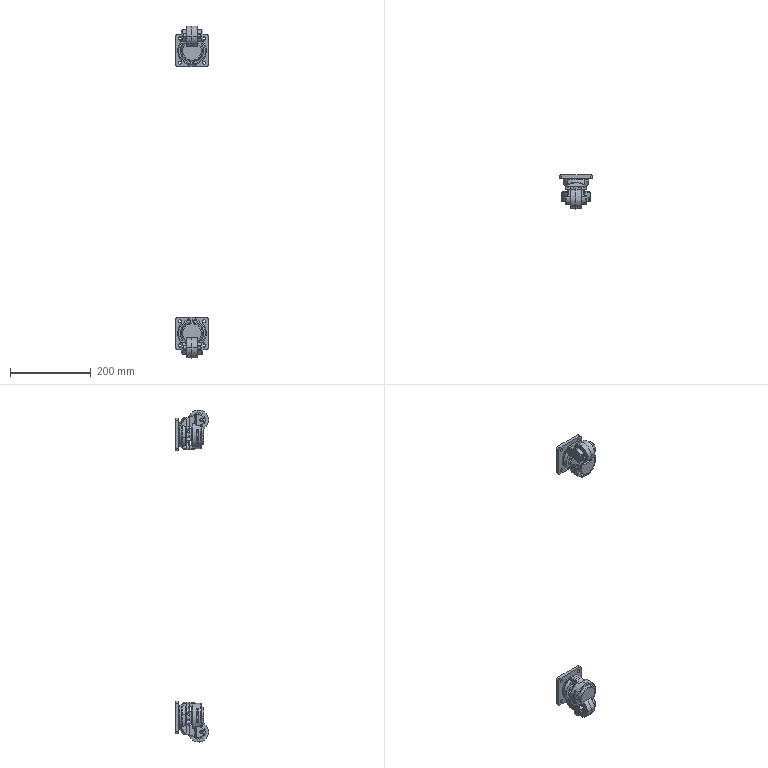Part | SolidWorks | 18 solids | 2054 faces | box 80 x 82.8 x 822 mm | volume 497420 mm3 | plane 874 | spline 448 | cylinder 438 | cone 158 | torus 88 | sphere 48 | commonest cylinder face diameters 2 x52 4 x48 68 x48 35 x32 10 x24 70 x24